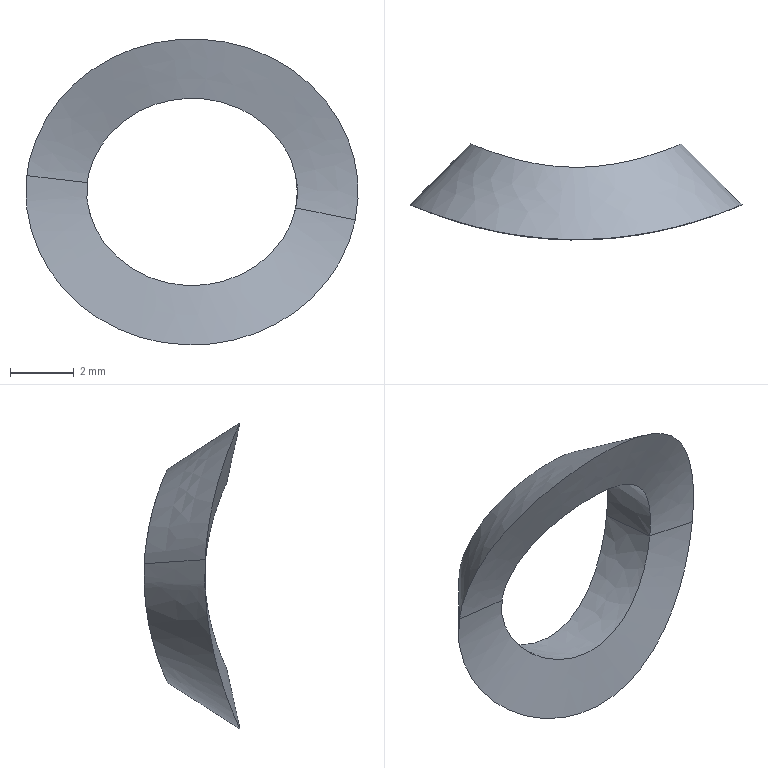Part | STEP file | 2026.6.15-Main Assembly图.sldasm-Part-285 | 1 solid | 6 faces | box 10.41 x 3.004 x 9.59 mm | volume 44.117 mm3 | spline 6